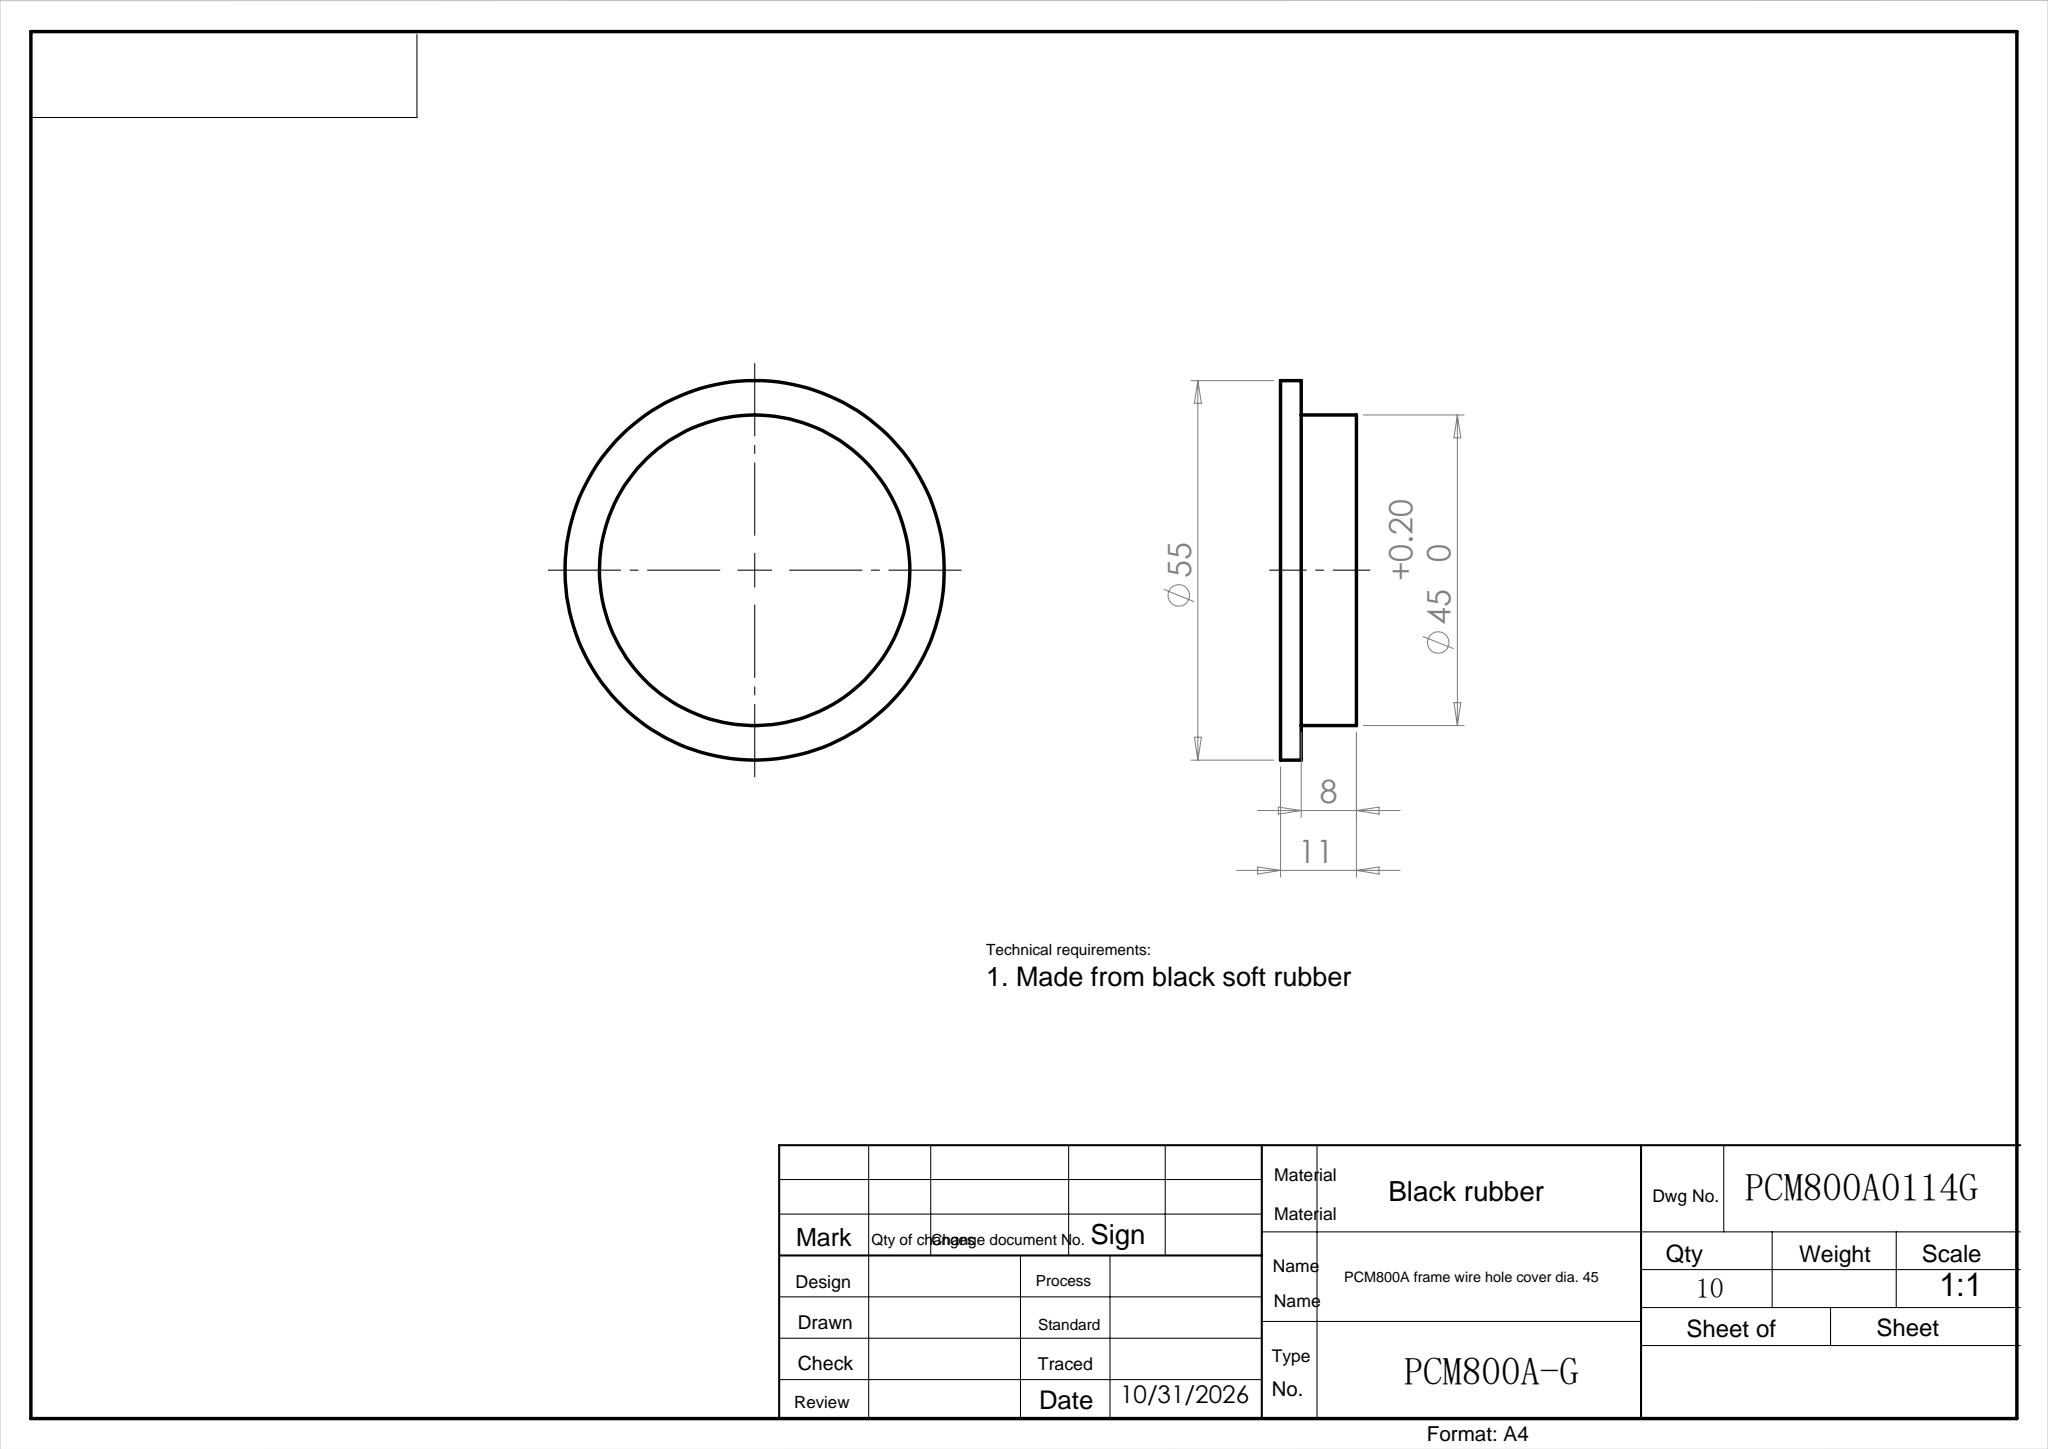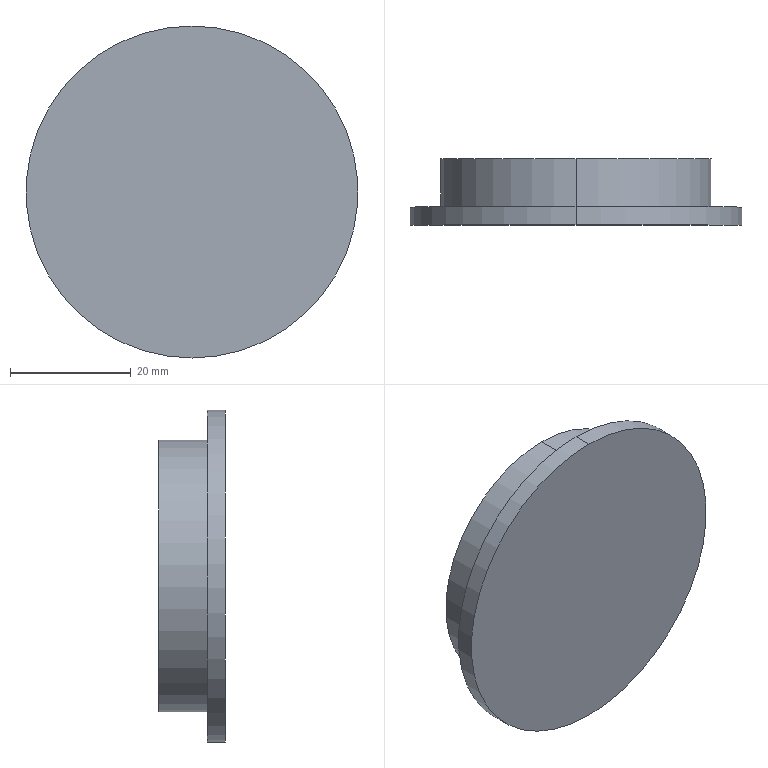Part | SolidWorks | features Revolution 1 | 1 solid | 7 faces | box 55 x 11 x 55 mm | volume 19851 mm3 | cylinder 4 | plane 3 | commonest cylinder face diameters 45 x2 55 x2
STEP:
#1=CARTESIAN_POINT('',(0.,11.,-22.5));
#2=VERTEX_POINT('',#1);
#3=CARTESIAN_POINT('',(0.,11.,22.5));
#4=VERTEX_POINT('',#3);
#5=CARTESIAN_POINT('',(0.,11.,0.));
#6=DIRECTION('',(0.,-1.,0.));
#7=DIRECTION('',(0.,0.,-1.));
#8=AXIS2_PLACEMENT_3D('',#5,#6,#7);
#9=CIRCLE('',#8,22.5);
#10=EDGE_CURVE('',#2,#4,#9,.T.);
#11=ORIENTED_EDGE('',*,*,#10,.T.);
#12=CARTESIAN_POINT('',(0.,3.,22.5));
#13=VERTEX_POINT('',#12);
#14=CARTESIAN_POINT('',(0.,0.,22.5));
#15=DIRECTION('',(0.,-1.,0.));
#16=VECTOR('',#15,1000.);
#17=LINE('',#14,#16);
#18=EDGE_CURVE('',#4,#13,#17,.T.);
#19=ORIENTED_EDGE('',*,*,#18,.T.);
#20=CARTESIAN_POINT('',(0.,3.,-22.5));
#21=VERTEX_POINT('',#20);
#22=CARTESIAN_POINT('',(0.,3.,0.));
#23=DIRECTION('',(0.,-1.,0.));
#24=DIRECTION('',(0.,0.,-1.));
#25=AXIS2_PLACEMENT_3D('',#22,#23,#24);
#26=CIRCLE('',#25,22.5);
#27=EDGE_CURVE('',#21,#13,#26,.T.);
#28=ORIENTED_EDGE('',*,*,#27,.F.);
#29=CARTESIAN_POINT('',(0.,0.,-22.5));
#30=DIRECTION('',(0.,-1.,0.));
#31=VECTOR('',#30,1000.);
#32=LINE('',#29,#31);
#33=EDGE_CURVE('',#2,#21,#32,.T.);
#34=ORIENTED_EDGE('',*,*,#33,.F.);
#35=EDGE_LOOP('',(#11,#19,#28,#34));
#36=FACE_OUTER_BOUND('',#35,.T.);
#37=CARTESIAN_POINT('',(0.,0.,0.));
#38=DIRECTION('',(0.,-1.,0.));
#39=DIRECTION('',(0.,0.,-1.));
#40=AXIS2_PLACEMENT_3D('',#37,#38,#39);
#41=CYLINDRICAL_SURFACE('',#40,22.5);
#42=ADVANCED_FACE('',(#36),#41,.T.);
#43=CARTESIAN_POINT('',(0.,3.,-27.5));
#44=VERTEX_POINT('',#43);
#45=CARTESIAN_POINT('',(0.,3.,27.5));
#46=VERTEX_POINT('',#45);
#47=CARTESIAN_POINT('',(0.,3.,0.));
#48=DIRECTION('',(0.,-1.,0.));
#49=DIRECTION('',(0.,0.,-1.));
#50=AXIS2_PLACEMENT_3D('',#47,#48,#49);
#51=CIRCLE('',#50,27.5);
#52=EDGE_CURVE('',#44,#46,#51,.T.);
#53=ORIENTED_EDGE('',*,*,#52,.T.);
#54=CARTESIAN_POINT('',(0.,0.,27.5));
#55=VERTEX_POINT('',#54);
#56=CARTESIAN_POINT('',(0.,0.,27.5));
#57=DIRECTION('',(0.,-1.,0.));
#58=VECTOR('',#57,1000.);
#59=LINE('',#56,#58);
#60=EDGE_CURVE('',#46,#55,#59,.T.);
#61=ORIENTED_EDGE('',*,*,#60,.T.);
#62=CARTESIAN_POINT('',(0.,0.,-27.5));
#63=VERTEX_POINT('',#62);
#64=CARTESIAN_POINT('',(0.,0.,0.));
#65=DIRECTION('',(0.,-1.,0.));
#66=DIRECTION('',(0.,0.,-1.));
#67=AXIS2_PLACEMENT_3D('',#64,#65,#66);
#68=CIRCLE('',#67,27.5);
#69=EDGE_CURVE('',#63,#55,#68,.T.);
#70=ORIENTED_EDGE('',*,*,#69,.F.);
#71=CARTESIAN_POINT('',(0.,0.,-27.5));
#72=DIRECTION('',(0.,-1.,0.));
#73=VECTOR('',#72,1000.);
#74=LINE('',#71,#73);
#75=EDGE_CURVE('',#44,#63,#74,.T.);
#76=ORIENTED_EDGE('',*,*,#75,.F.);
#77=EDGE_LOOP('',(#53,#61,#70,#76));
#78=FACE_OUTER_BOUND('',#77,.T.);
#79=CARTESIAN_POINT('',(0.,0.,0.));
#80=DIRECTION('',(0.,-1.,0.));
#81=DIRECTION('',(0.,0.,-1.));
#82=AXIS2_PLACEMENT_3D('',#79,#80,#81);
#83=CYLINDRICAL_SURFACE('',#82,27.5);
#84=ADVANCED_FACE('',(#78),#83,.T.);
#85=ORIENTED_EDGE('',*,*,#69,.T.);
#86=CARTESIAN_POINT('',(0.,0.,0.));
#87=DIRECTION('',(0.,-1.,0.));
#88=DIRECTION('',(0.,0.,-1.));
#89=AXIS2_PLACEMENT_3D('',#86,#87,#88);
#90=CIRCLE('',#89,27.5);
#91=EDGE_CURVE('',#55,#63,#90,.T.);
#92=ORIENTED_EDGE('',*,*,#91,.T.);
#93=EDGE_LOOP('',(#85,#92));
#94=FACE_OUTER_BOUND('',#93,.T.);
#95=CARTESIAN_POINT('',(0.,0.,0.));
#96=DIRECTION('',(0.,1.,0.));
#97=DIRECTION('',(0.,0.,1.));
#98=AXIS2_PLACEMENT_3D('',#95,#96,#97);
#99=PLANE('',#98);
#100=ADVANCED_FACE('',(#94),#99,.F.);
#101=ORIENTED_EDGE('',*,*,#60,.F.);
#102=CARTESIAN_POINT('',(0.,3.,0.));
#103=DIRECTION('',(0.,-1.,0.));
#104=DIRECTION('',(0.,0.,-1.));
#105=AXIS2_PLACEMENT_3D('',#102,#103,#104);
#106=CIRCLE('',#105,27.5);
#107=EDGE_CURVE('',#46,#44,#106,.T.);
#108=ORIENTED_EDGE('',*,*,#107,.T.);
#109=ORIENTED_EDGE('',*,*,#75,.T.);
#110=ORIENTED_EDGE('',*,*,#91,.F.);
#111=EDGE_LOOP('',(#101,#108,#109,#110));
#112=FACE_OUTER_BOUND('',#111,.T.);
#113=CARTESIAN_POINT('',(0.,0.,0.));
#114=DIRECTION('',(0.,-1.,0.));
#115=DIRECTION('',(0.,0.,-1.));
#116=AXIS2_PLACEMENT_3D('',#113,#114,#115);
#117=CYLINDRICAL_SURFACE('',#116,27.5);
#118=ADVANCED_FACE('',(#112),#117,.T.);
#119=ORIENTED_EDGE('',*,*,#52,.F.);
#120=ORIENTED_EDGE('',*,*,#107,.F.);
#121=EDGE_LOOP('',(#119,#120));
#122=FACE_OUTER_BOUND('',#121,.T.);
#123=ORIENTED_EDGE('',*,*,#27,.T.);
#124=CARTESIAN_POINT('',(0.,3.,0.));
#125=DIRECTION('',(0.,-1.,0.));
#126=DIRECTION('',(0.,0.,-1.));
#127=AXIS2_PLACEMENT_3D('',#124,#125,#126);
#128=CIRCLE('',#127,22.5);
#129=EDGE_CURVE('',#13,#21,#128,.T.);
#130=ORIENTED_EDGE('',*,*,#129,.T.);
#131=EDGE_LOOP('',(#123,#130));
#132=FACE_BOUND('',#131,.T.);
#133=CARTESIAN_POINT('',(27.5,3.,0.));
#134=DIRECTION('',(0.,-1.,0.));
#135=DIRECTION('',(0.,0.,-1.));
#136=AXIS2_PLACEMENT_3D('',#133,#134,#135);
#137=PLANE('',#136);
#138=ADVANCED_FACE('',(#122,#132),#137,.F.);
#139=ORIENTED_EDGE('',*,*,#18,.F.);
#140=CARTESIAN_POINT('',(0.,11.,0.));
#141=DIRECTION('',(0.,-1.,0.));
#142=DIRECTION('',(0.,0.,-1.));
#143=AXIS2_PLACEMENT_3D('',#140,#141,#142);
#144=CIRCLE('',#143,22.5);
#145=EDGE_CURVE('',#4,#2,#144,.T.);
#146=ORIENTED_EDGE('',*,*,#145,.T.);
#147=ORIENTED_EDGE('',*,*,#33,.T.);
#148=ORIENTED_EDGE('',*,*,#129,.F.);
#149=EDGE_LOOP('',(#139,#146,#147,#148));
#150=FACE_OUTER_BOUND('',#149,.T.);
#151=CARTESIAN_POINT('',(0.,0.,0.));
#152=DIRECTION('',(0.,-1.,0.));
#153=DIRECTION('',(0.,0.,-1.));
#154=AXIS2_PLACEMENT_3D('',#151,#152,#153);
#155=CYLINDRICAL_SURFACE('',#154,22.5);
#156=ADVANCED_FACE('',(#150),#155,.T.);
#157=ORIENTED_EDGE('',*,*,#10,.F.);
#158=ORIENTED_EDGE('',*,*,#145,.F.);
#159=EDGE_LOOP('',(#157,#158));
#160=FACE_OUTER_BOUND('',#159,.T.);
#161=CARTESIAN_POINT('',(22.5,11.,0.));
#162=DIRECTION('',(0.,-1.,0.));
#163=DIRECTION('',(0.,0.,-1.));
#164=AXIS2_PLACEMENT_3D('',#161,#162,#163);
#165=PLANE('',#164);
#166=ADVANCED_FACE('',(#160),#165,.F.);
#167=CLOSED_SHELL('',(#42,#84,#100,#118,#138,#156,#166));
#168=MANIFOLD_SOLID_BREP('',#167);
#169=CARTESIAN_POINT('',(0.,0.,0.));
#170=DIRECTION('',(0.,0.,1.));
#171=DIRECTION('',(1.,0.,0.));
#172=AXIS2_PLACEMENT_3D('',#169,#170,#171);
#173=(LENGTH_UNIT()NAMED_UNIT(*)SI_UNIT(.MILLI.,.METRE.));
#174=UNCERTAINTY_MEASURE_WITH_UNIT(LENGTH_MEASURE(0.00001),#173,'','');
#175=(NAMED_UNIT(*)PLANE_ANGLE_UNIT()SI_UNIT($,.RADIAN.));
#176=(NAMED_UNIT(*)SI_UNIT($,.STERADIAN.)SOLID_ANGLE_UNIT());
#177=(GEOMETRIC_REPRESENTATION_CONTEXT(3)GLOBAL_UNCERTAINTY_ASSIGNED_CONTEXT((#174))GLOBAL_UNIT_ASSIGNED_CONTEXT((#173,#175,#176))REPRESENTATION_CONTEXT('',''));
#178=ADVANCED_BREP_SHAPE_REPRESENTATION('',(#168,#172),#177);